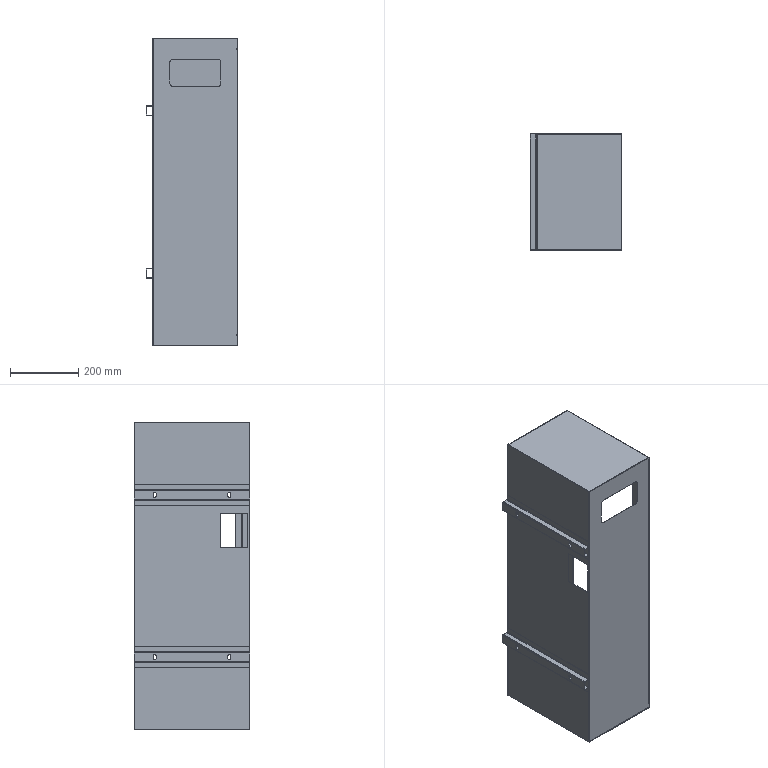Part | SolidWorks | features MirrorCompFeat 1, ReferencePattern 1 | 5 solids | 295 faces | box 270 x 340 x 900 mm | volume 1657617 mm3 | plane 228 | cylinder 67 | commonest cylinder face diameters 2 x22 5 x22 20 x12 9 x8 40 x3